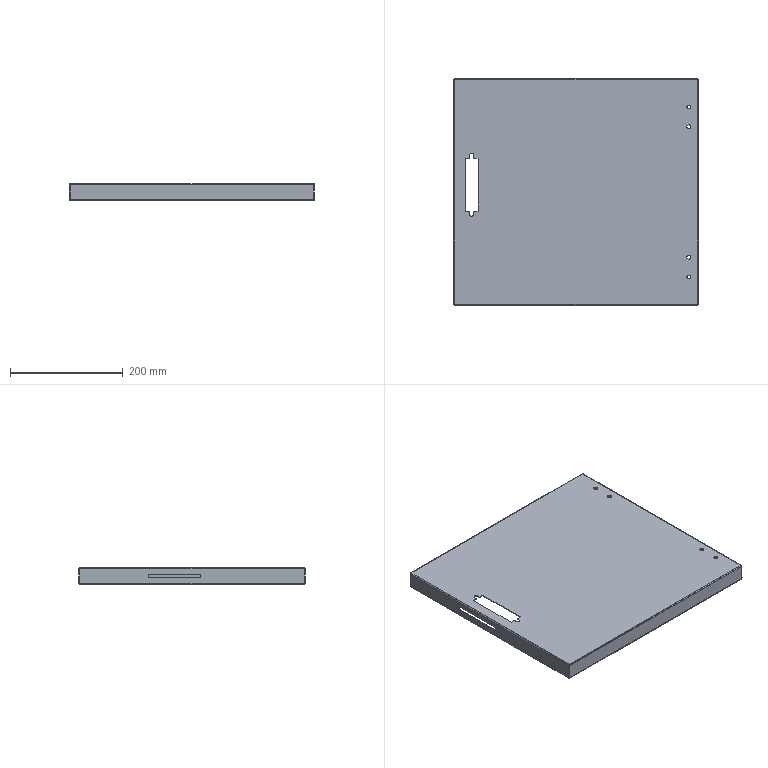Part | 1 solid | 95 faces | box 435 x 402 x 30 mm | volume 282319 mm3 | plane 50 | cylinder 29 | spline 16 | commonest cylinder face diameters 7 x13 1.473 x8 3.873 x8